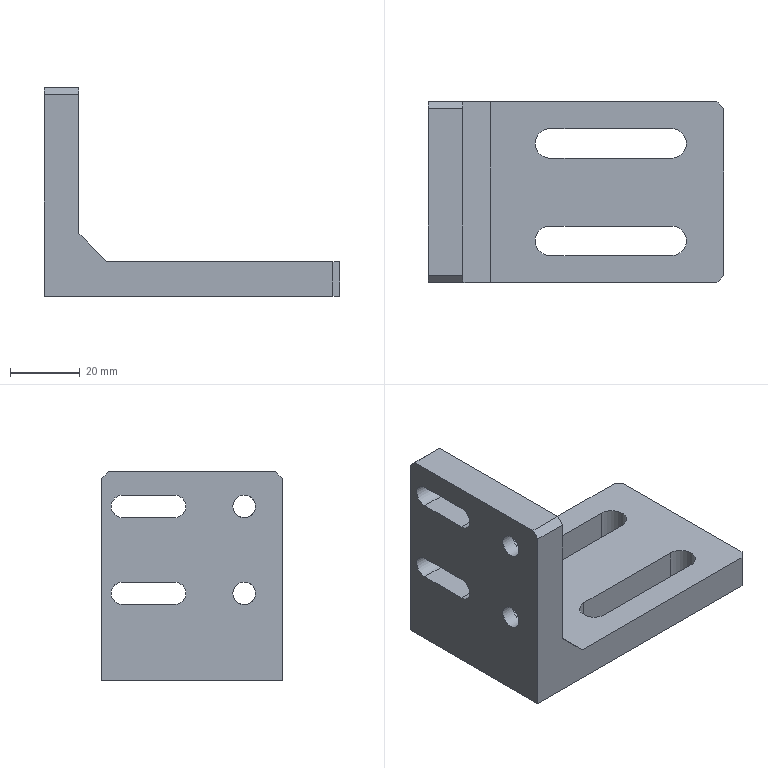Part | STEP file | Tube necking machine_id650_x_t | 1 solid | 35 faces | box 85 x 52 x 60 mm | volume 60680 mm3 | plane 23 | cylinder 12 | commonest cylinder face diameters 6.5 x6 8.5 x4 11 x2